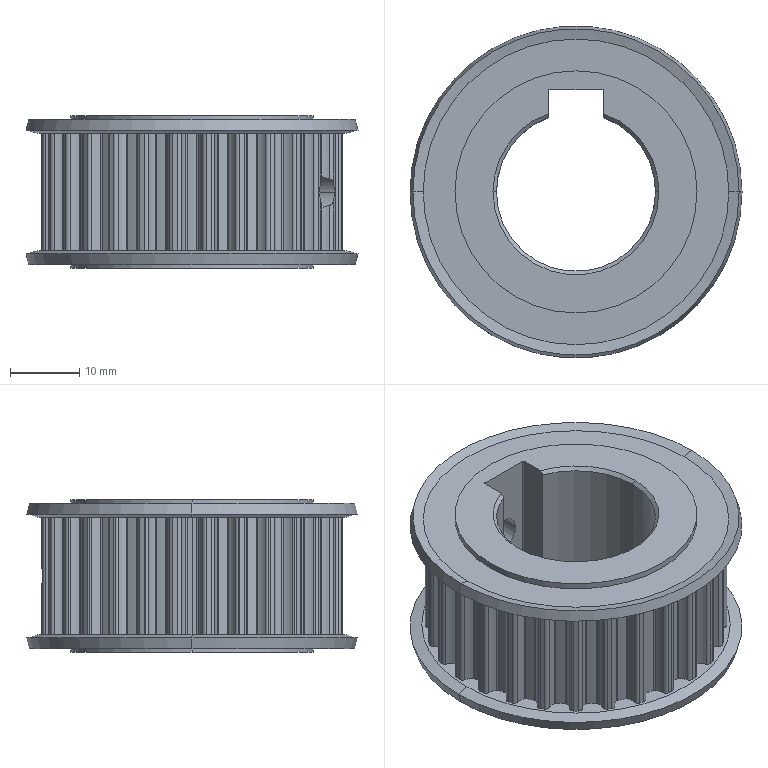Part | STEP file | EBJ21-S5M150-28-A-N-d23^Mechanical tensioner (pay-off) | 1 solid | 304 faces | box 48 x 48 x 22 mm | volume 20519 mm3 | cylinder 277 | cone 18 | plane 9 | commonest cylinder face diameters 1.1 x72 0.5 x69 6.55 x64 40.06 x31 43.6 x28 4.917 x4